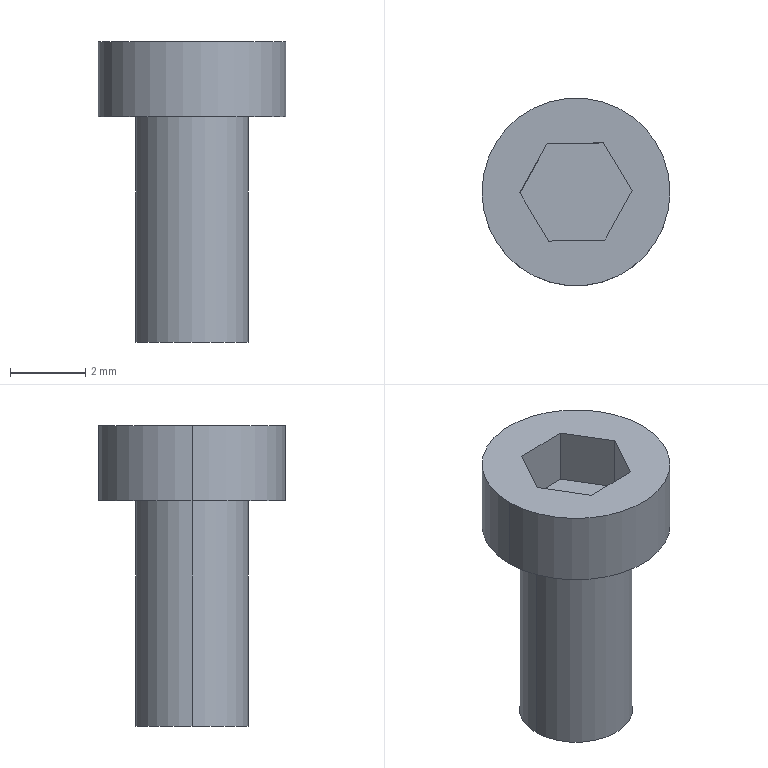Part | SolidWorks | features Cut 1, Extrusion 1, ICE 1 | 1 solid | 14 faces | box 5 x 5 x 8 mm | volume 72.989 mm3 | plane 10 | cylinder 4 | commonest cylinder face diameters 3 x2 5 x2
STEP:
#1=CARTESIAN_POINT('',(2.5,0.,2.));
#2=VERTEX_POINT('',#1);
#3=CARTESIAN_POINT('',(-2.5,0.,2.));
#4=VERTEX_POINT('',#3);
#5=CARTESIAN_POINT('',(0.,0.,2.));
#6=DIRECTION('',(0.,0.,1.));
#7=DIRECTION('',(1.,0.,0.));
#8=AXIS2_PLACEMENT_3D('',#5,#6,#7);
#9=CIRCLE('',#8,2.5);
#10=EDGE_CURVE('',#2,#4,#9,.T.);
#11=ORIENTED_EDGE('',*,*,#10,.F.);
#12=CARTESIAN_POINT('',(2.5,0.,0.));
#13=VERTEX_POINT('',#12);
#14=CARTESIAN_POINT('',(2.5,0.,2.));
#15=DIRECTION('',(0.,0.,-1.));
#16=VECTOR('',#15,1000.);
#17=LINE('',#14,#16);
#18=EDGE_CURVE('',#2,#13,#17,.T.);
#19=ORIENTED_EDGE('',*,*,#18,.T.);
#20=CARTESIAN_POINT('',(-2.5,0.,0.));
#21=VERTEX_POINT('',#20);
#22=CARTESIAN_POINT('',(0.,0.,0.));
#23=DIRECTION('',(0.,0.,1.));
#24=DIRECTION('',(1.,0.,0.));
#25=AXIS2_PLACEMENT_3D('',#22,#23,#24);
#26=CIRCLE('',#25,2.5);
#27=EDGE_CURVE('',#13,#21,#26,.T.);
#28=ORIENTED_EDGE('',*,*,#27,.T.);
#29=CARTESIAN_POINT('',(-2.5,0.,2.));
#30=DIRECTION('',(0.,0.,-1.));
#31=VECTOR('',#30,1000.);
#32=LINE('',#29,#31);
#33=EDGE_CURVE('',#4,#21,#32,.T.);
#34=ORIENTED_EDGE('',*,*,#33,.F.);
#35=EDGE_LOOP('',(#11,#19,#28,#34));
#36=FACE_OUTER_BOUND('',#35,.T.);
#37=CARTESIAN_POINT('',(0.,0.,2.));
#38=DIRECTION('',(0.,0.,-1.));
#39=DIRECTION('',(-1.,0.,0.));
#40=AXIS2_PLACEMENT_3D('',#37,#38,#39);
#41=CYLINDRICAL_SURFACE('',#40,2.5);
#42=ADVANCED_FACE('',(#36),#41,.T.);
#43=CARTESIAN_POINT('',(1.5,0.,-6.));
#44=VERTEX_POINT('',#43);
#45=CARTESIAN_POINT('',(-1.5,0.,-6.));
#46=VERTEX_POINT('',#45);
#47=CARTESIAN_POINT('',(0.,0.,-6.));
#48=DIRECTION('',(0.,0.,1.));
#49=DIRECTION('',(1.,0.,0.));
#50=AXIS2_PLACEMENT_3D('',#47,#48,#49);
#51=CIRCLE('',#50,1.5);
#52=EDGE_CURVE('',#44,#46,#51,.T.);
#53=ORIENTED_EDGE('',*,*,#52,.T.);
#54=CARTESIAN_POINT('',(-1.5,0.,0.));
#55=VERTEX_POINT('',#54);
#56=CARTESIAN_POINT('',(-1.5,0.,-6.));
#57=DIRECTION('',(0.,0.,1.));
#58=VECTOR('',#57,1000.);
#59=LINE('',#56,#58);
#60=EDGE_CURVE('',#46,#55,#59,.T.);
#61=ORIENTED_EDGE('',*,*,#60,.T.);
#62=CARTESIAN_POINT('',(1.5,0.,0.));
#63=VERTEX_POINT('',#62);
#64=CARTESIAN_POINT('',(0.,0.,0.));
#65=DIRECTION('',(0.,0.,1.));
#66=DIRECTION('',(1.,0.,0.));
#67=AXIS2_PLACEMENT_3D('',#64,#65,#66);
#68=CIRCLE('',#67,1.5);
#69=EDGE_CURVE('',#63,#55,#68,.T.);
#70=ORIENTED_EDGE('',*,*,#69,.F.);
#71=CARTESIAN_POINT('',(1.5,0.,-6.));
#72=DIRECTION('',(0.,0.,1.));
#73=VECTOR('',#72,1000.);
#74=LINE('',#71,#73);
#75=EDGE_CURVE('',#44,#63,#74,.T.);
#76=ORIENTED_EDGE('',*,*,#75,.F.);
#77=EDGE_LOOP('',(#53,#61,#70,#76));
#78=FACE_OUTER_BOUND('',#77,.T.);
#79=CARTESIAN_POINT('',(0.,0.,-6.));
#80=DIRECTION('',(0.,0.,1.));
#81=DIRECTION('',(1.,0.,0.));
#82=AXIS2_PLACEMENT_3D('',#79,#80,#81);
#83=CYLINDRICAL_SURFACE('',#82,1.5);
#84=ADVANCED_FACE('',(#78),#83,.T.);
#85=ORIENTED_EDGE('',*,*,#60,.F.);
#86=CARTESIAN_POINT('',(0.,0.,-6.));
#87=DIRECTION('',(0.,0.,1.));
#88=DIRECTION('',(1.,0.,0.));
#89=AXIS2_PLACEMENT_3D('',#86,#87,#88);
#90=CIRCLE('',#89,1.5);
#91=EDGE_CURVE('',#46,#44,#90,.T.);
#92=ORIENTED_EDGE('',*,*,#91,.T.);
#93=ORIENTED_EDGE('',*,*,#75,.T.);
#94=CARTESIAN_POINT('',(0.,0.,0.));
#95=DIRECTION('',(0.,0.,1.));
#96=DIRECTION('',(1.,0.,0.));
#97=AXIS2_PLACEMENT_3D('',#94,#95,#96);
#98=CIRCLE('',#97,1.5);
#99=EDGE_CURVE('',#55,#63,#98,.T.);
#100=ORIENTED_EDGE('',*,*,#99,.F.);
#101=EDGE_LOOP('',(#85,#92,#93,#100));
#102=FACE_OUTER_BOUND('',#101,.T.);
#103=CARTESIAN_POINT('',(0.,0.,-6.));
#104=DIRECTION('',(0.,0.,1.));
#105=DIRECTION('',(1.,0.,0.));
#106=AXIS2_PLACEMENT_3D('',#103,#104,#105);
#107=CYLINDRICAL_SURFACE('',#106,1.5);
#108=ADVANCED_FACE('',(#102),#107,.T.);
#109=ORIENTED_EDGE('',*,*,#52,.F.);
#110=ORIENTED_EDGE('',*,*,#91,.F.);
#111=EDGE_LOOP('',(#109,#110));
#112=FACE_OUTER_BOUND('',#111,.T.);
#113=CARTESIAN_POINT('',(0.,0.,-6.));
#114=DIRECTION('',(0.,0.,1.));
#115=DIRECTION('',(1.,0.,0.));
#116=AXIS2_PLACEMENT_3D('',#113,#114,#115);
#117=PLANE('',#116);
#118=ADVANCED_FACE('',(#112),#117,.F.);
#119=ORIENTED_EDGE('',*,*,#18,.F.);
#120=CARTESIAN_POINT('',(0.,0.,2.));
#121=DIRECTION('',(0.,0.,1.));
#122=DIRECTION('',(1.,0.,0.));
#123=AXIS2_PLACEMENT_3D('',#120,#121,#122);
#124=CIRCLE('',#123,2.5);
#125=EDGE_CURVE('',#4,#2,#124,.T.);
#126=ORIENTED_EDGE('',*,*,#125,.F.);
#127=ORIENTED_EDGE('',*,*,#33,.T.);
#128=CARTESIAN_POINT('',(0.,0.,0.));
#129=DIRECTION('',(0.,0.,1.));
#130=DIRECTION('',(1.,0.,0.));
#131=AXIS2_PLACEMENT_3D('',#128,#129,#130);
#132=CIRCLE('',#131,2.5);
#133=EDGE_CURVE('',#21,#13,#132,.T.);
#134=ORIENTED_EDGE('',*,*,#133,.T.);
#135=EDGE_LOOP('',(#119,#126,#127,#134));
#136=FACE_OUTER_BOUND('',#135,.T.);
#137=CARTESIAN_POINT('',(0.,0.,2.));
#138=DIRECTION('',(0.,0.,-1.));
#139=DIRECTION('',(-1.,0.,0.));
#140=AXIS2_PLACEMENT_3D('',#137,#138,#139);
#141=CYLINDRICAL_SURFACE('',#140,2.5);
#142=ADVANCED_FACE('',(#136),#141,.T.);
#143=CARTESIAN_POINT('',(1.493,0.02809,2.));
#144=VERTEX_POINT('',#143);
#145=CARTESIAN_POINT('',(0.7223,1.307,2.));
#146=VERTEX_POINT('',#145);
#147=CARTESIAN_POINT('',(1.493,0.02809,2.));
#148=DIRECTION('',(-0.5162,0.8565,0.));
#149=VECTOR('',#148,1000.);
#150=LINE('',#147,#149);
#151=EDGE_CURVE('',#144,#146,#150,.T.);
#152=ORIENTED_EDGE('',*,*,#151,.F.);
#153=CARTESIAN_POINT('',(0.7709,-1.279,2.));
#154=VERTEX_POINT('',#153);
#155=CARTESIAN_POINT('',(0.7709,-1.279,2.));
#156=DIRECTION('',(0.4836,0.8753,0.));
#157=VECTOR('',#156,1000.);
#158=LINE('',#155,#157);
#159=EDGE_CURVE('',#154,#144,#158,.T.);
#160=ORIENTED_EDGE('',*,*,#159,.F.);
#161=CARTESIAN_POINT('',(-0.7223,-1.307,2.));
#162=VERTEX_POINT('',#161);
#163=CARTESIAN_POINT('',(-0.7223,-1.307,2.));
#164=DIRECTION('',(0.9998,0.01881,0.));
#165=VECTOR('',#164,1000.);
#166=LINE('',#163,#165);
#167=EDGE_CURVE('',#162,#154,#166,.T.);
#168=ORIENTED_EDGE('',*,*,#167,.F.);
#169=CARTESIAN_POINT('',(-1.493,-0.02809,2.));
#170=VERTEX_POINT('',#169);
#171=CARTESIAN_POINT('',(-1.493,-0.02809,2.));
#172=DIRECTION('',(0.5162,-0.8565,0.));
#173=VECTOR('',#172,1000.);
#174=LINE('',#171,#173);
#175=EDGE_CURVE('',#170,#162,#174,.T.);
#176=ORIENTED_EDGE('',*,*,#175,.F.);
#177=CARTESIAN_POINT('',(-0.7709,1.279,2.));
#178=VERTEX_POINT('',#177);
#179=CARTESIAN_POINT('',(-0.7709,1.279,2.));
#180=DIRECTION('',(-0.4836,-0.8753,0.));
#181=VECTOR('',#180,1000.);
#182=LINE('',#179,#181);
#183=EDGE_CURVE('',#178,#170,#182,.T.);
#184=ORIENTED_EDGE('',*,*,#183,.F.);
#185=CARTESIAN_POINT('',(0.7223,1.307,2.));
#186=DIRECTION('',(-0.9998,-0.01881,0.));
#187=VECTOR('',#186,1000.);
#188=LINE('',#185,#187);
#189=EDGE_CURVE('',#146,#178,#188,.T.);
#190=ORIENTED_EDGE('',*,*,#189,.F.);
#191=EDGE_LOOP('',(#152,#160,#168,#176,#184,#190));
#192=FACE_BOUND('',#191,.T.);
#193=ORIENTED_EDGE('',*,*,#125,.T.);
#194=ORIENTED_EDGE('',*,*,#10,.T.);
#195=EDGE_LOOP('',(#193,#194));
#196=FACE_OUTER_BOUND('',#195,.T.);
#197=CARTESIAN_POINT('',(0.,0.,2.));
#198=DIRECTION('',(0.,0.,1.));
#199=DIRECTION('',(1.,0.,0.));
#200=AXIS2_PLACEMENT_3D('',#197,#198,#199);
#201=PLANE('',#200);
#202=ADVANCED_FACE('',(#192,#196),#201,.T.);
#203=ORIENTED_EDGE('',*,*,#69,.T.);
#204=ORIENTED_EDGE('',*,*,#99,.T.);
#205=EDGE_LOOP('',(#203,#204));
#206=FACE_BOUND('',#205,.T.);
#207=ORIENTED_EDGE('',*,*,#133,.F.);
#208=ORIENTED_EDGE('',*,*,#27,.F.);
#209=EDGE_LOOP('',(#207,#208));
#210=FACE_OUTER_BOUND('',#209,.T.);
#211=CARTESIAN_POINT('',(0.,0.,0.));
#212=DIRECTION('',(0.,0.,1.));
#213=DIRECTION('',(1.,0.,0.));
#214=AXIS2_PLACEMENT_3D('',#211,#212,#213);
#215=PLANE('',#214);
#216=ADVANCED_FACE('',(#206,#210),#215,.F.);
#217=ORIENTED_EDGE('',*,*,#151,.T.);
#218=CARTESIAN_POINT('',(0.7223,1.307,0.5));
#219=VERTEX_POINT('',#218);
#220=CARTESIAN_POINT('',(0.7223,1.307,0.5));
#221=DIRECTION('',(0.,0.,1.));
#222=VECTOR('',#221,1000.);
#223=LINE('',#220,#222);
#224=EDGE_CURVE('',#219,#146,#223,.T.);
#225=ORIENTED_EDGE('',*,*,#224,.F.);
#226=CARTESIAN_POINT('',(1.493,0.02809,0.5));
#227=VERTEX_POINT('',#226);
#228=CARTESIAN_POINT('',(1.493,0.02809,0.5));
#229=DIRECTION('',(-0.5162,0.8565,0.));
#230=VECTOR('',#229,1000.);
#231=LINE('',#228,#230);
#232=EDGE_CURVE('',#227,#219,#231,.T.);
#233=ORIENTED_EDGE('',*,*,#232,.F.);
#234=CARTESIAN_POINT('',(1.493,0.02809,0.5));
#235=DIRECTION('',(0.,0.,1.));
#236=VECTOR('',#235,1000.);
#237=LINE('',#234,#236);
#238=EDGE_CURVE('',#227,#144,#237,.T.);
#239=ORIENTED_EDGE('',*,*,#238,.T.);
#240=EDGE_LOOP('',(#217,#225,#233,#239));
#241=FACE_OUTER_BOUND('',#240,.T.);
#242=CARTESIAN_POINT('',(1.493,0.02809,0.5));
#243=DIRECTION('',(0.8565,0.5162,0.));
#244=DIRECTION('',(-0.5162,0.8565,0.));
#245=AXIS2_PLACEMENT_3D('',#242,#243,#244);
#246=PLANE('',#245);
#247=ADVANCED_FACE('',(#241),#246,.F.);
#248=ORIENTED_EDGE('',*,*,#159,.T.);
#249=ORIENTED_EDGE('',*,*,#238,.F.);
#250=CARTESIAN_POINT('',(0.7709,-1.279,0.5));
#251=VERTEX_POINT('',#250);
#252=CARTESIAN_POINT('',(0.7709,-1.279,0.5));
#253=DIRECTION('',(0.4836,0.8753,0.));
#254=VECTOR('',#253,1000.);
#255=LINE('',#252,#254);
#256=EDGE_CURVE('',#251,#227,#255,.T.);
#257=ORIENTED_EDGE('',*,*,#256,.F.);
#258=CARTESIAN_POINT('',(0.7709,-1.279,0.5));
#259=DIRECTION('',(0.,0.,1.));
#260=VECTOR('',#259,1000.);
#261=LINE('',#258,#260);
#262=EDGE_CURVE('',#251,#154,#261,.T.);
#263=ORIENTED_EDGE('',*,*,#262,.T.);
#264=EDGE_LOOP('',(#248,#249,#257,#263));
#265=FACE_OUTER_BOUND('',#264,.T.);
#266=CARTESIAN_POINT('',(0.7709,-1.279,0.5));
#267=DIRECTION('',(0.8753,-0.4836,0.));
#268=DIRECTION('',(0.4836,0.8753,0.));
#269=AXIS2_PLACEMENT_3D('',#266,#267,#268);
#270=PLANE('',#269);
#271=ADVANCED_FACE('',(#265),#270,.F.);
#272=ORIENTED_EDGE('',*,*,#167,.T.);
#273=ORIENTED_EDGE('',*,*,#262,.F.);
#274=CARTESIAN_POINT('',(-0.7223,-1.307,0.5));
#275=VERTEX_POINT('',#274);
#276=CARTESIAN_POINT('',(-0.7223,-1.307,0.5));
#277=DIRECTION('',(0.9998,0.01881,0.));
#278=VECTOR('',#277,1000.);
#279=LINE('',#276,#278);
#280=EDGE_CURVE('',#275,#251,#279,.T.);
#281=ORIENTED_EDGE('',*,*,#280,.F.);
#282=CARTESIAN_POINT('',(-0.7223,-1.307,0.5));
#283=DIRECTION('',(0.,0.,1.));
#284=VECTOR('',#283,1000.);
#285=LINE('',#282,#284);
#286=EDGE_CURVE('',#275,#162,#285,.T.);
#287=ORIENTED_EDGE('',*,*,#286,.T.);
#288=EDGE_LOOP('',(#272,#273,#281,#287));
#289=FACE_OUTER_BOUND('',#288,.T.);
#290=CARTESIAN_POINT('',(-0.7223,-1.307,0.5));
#291=DIRECTION('',(0.01881,-0.9998,0.));
#292=DIRECTION('',(0.9998,0.01881,0.));
#293=AXIS2_PLACEMENT_3D('',#290,#291,#292);
#294=PLANE('',#293);
#295=ADVANCED_FACE('',(#289),#294,.F.);
#296=ORIENTED_EDGE('',*,*,#175,.T.);
#297=ORIENTED_EDGE('',*,*,#286,.F.);
#298=CARTESIAN_POINT('',(-1.493,-0.02809,0.5));
#299=VERTEX_POINT('',#298);
#300=CARTESIAN_POINT('',(-1.493,-0.02809,0.5));
#301=DIRECTION('',(0.5162,-0.8565,0.));
#302=VECTOR('',#301,1000.);
#303=LINE('',#300,#302);
#304=EDGE_CURVE('',#299,#275,#303,.T.);
#305=ORIENTED_EDGE('',*,*,#304,.F.);
#306=CARTESIAN_POINT('',(-1.493,-0.02809,0.5));
#307=DIRECTION('',(0.,0.,1.));
#308=VECTOR('',#307,1000.);
#309=LINE('',#306,#308);
#310=EDGE_CURVE('',#299,#170,#309,.T.);
#311=ORIENTED_EDGE('',*,*,#310,.T.);
#312=EDGE_LOOP('',(#296,#297,#305,#311));
#313=FACE_OUTER_BOUND('',#312,.T.);
#314=CARTESIAN_POINT('',(-1.493,-0.02809,0.5));
#315=DIRECTION('',(-0.8565,-0.5162,0.));
#316=DIRECTION('',(0.5162,-0.8565,0.));
#317=AXIS2_PLACEMENT_3D('',#314,#315,#316);
#318=PLANE('',#317);
#319=ADVANCED_FACE('',(#313),#318,.F.);
#320=ORIENTED_EDGE('',*,*,#183,.T.);
#321=ORIENTED_EDGE('',*,*,#310,.F.);
#322=CARTESIAN_POINT('',(-0.7709,1.279,0.5));
#323=VERTEX_POINT('',#322);
#324=CARTESIAN_POINT('',(-0.7709,1.279,0.5));
#325=DIRECTION('',(-0.4836,-0.8753,0.));
#326=VECTOR('',#325,1000.);
#327=LINE('',#324,#326);
#328=EDGE_CURVE('',#323,#299,#327,.T.);
#329=ORIENTED_EDGE('',*,*,#328,.F.);
#330=CARTESIAN_POINT('',(-0.7709,1.279,0.5));
#331=DIRECTION('',(0.,0.,1.));
#332=VECTOR('',#331,1000.);
#333=LINE('',#330,#332);
#334=EDGE_CURVE('',#323,#178,#333,.T.);
#335=ORIENTED_EDGE('',*,*,#334,.T.);
#336=EDGE_LOOP('',(#320,#321,#329,#335));
#337=FACE_OUTER_BOUND('',#336,.T.);
#338=CARTESIAN_POINT('',(-0.7709,1.279,0.5));
#339=DIRECTION('',(-0.8753,0.4836,0.));
#340=DIRECTION('',(-0.4836,-0.8753,0.));
#341=AXIS2_PLACEMENT_3D('',#338,#339,#340);
#342=PLANE('',#341);
#343=ADVANCED_FACE('',(#337),#342,.F.);
#344=ORIENTED_EDGE('',*,*,#189,.T.);
#345=ORIENTED_EDGE('',*,*,#334,.F.);
#346=CARTESIAN_POINT('',(0.7223,1.307,0.5));
#347=DIRECTION('',(-0.9998,-0.01881,0.));
#348=VECTOR('',#347,1000.);
#349=LINE('',#346,#348);
#350=EDGE_CURVE('',#219,#323,#349,.T.);
#351=ORIENTED_EDGE('',*,*,#350,.F.);
#352=ORIENTED_EDGE('',*,*,#224,.T.);
#353=EDGE_LOOP('',(#344,#345,#351,#352));
#354=FACE_OUTER_BOUND('',#353,.T.);
#355=CARTESIAN_POINT('',(0.7223,1.307,0.5));
#356=DIRECTION('',(-0.01881,0.9998,0.));
#357=DIRECTION('',(-0.9998,-0.01881,0.));
#358=AXIS2_PLACEMENT_3D('',#355,#356,#357);
#359=PLANE('',#358);
#360=ADVANCED_FACE('',(#354),#359,.F.);
#361=ORIENTED_EDGE('',*,*,#232,.T.);
#362=ORIENTED_EDGE('',*,*,#350,.T.);
#363=ORIENTED_EDGE('',*,*,#328,.T.);
#364=ORIENTED_EDGE('',*,*,#304,.T.);
#365=ORIENTED_EDGE('',*,*,#280,.T.);
#366=ORIENTED_EDGE('',*,*,#256,.T.);
#367=EDGE_LOOP('',(#361,#362,#363,#364,#365,#366));
#368=FACE_OUTER_BOUND('',#367,.T.);
#369=CARTESIAN_POINT('',(0.,0.,0.5));
#370=DIRECTION('',(0.,0.,1.));
#371=DIRECTION('',(1.,0.,0.));
#372=AXIS2_PLACEMENT_3D('',#369,#370,#371);
#373=PLANE('',#372);
#374=ADVANCED_FACE('',(#368),#373,.T.);
#375=CLOSED_SHELL('',(#42,#84,#108,#118,#142,#202,#216,#247,#271,#295,#319,#343,#360,#374));
#376=MANIFOLD_SOLID_BREP('',#375);
#377=CARTESIAN_POINT('',(0.,0.,0.));
#378=DIRECTION('',(0.,0.,1.));
#379=DIRECTION('',(1.,0.,0.));
#380=AXIS2_PLACEMENT_3D('',#377,#378,#379);
#381=(LENGTH_UNIT()NAMED_UNIT(*)SI_UNIT(.MILLI.,.METRE.));
#382=UNCERTAINTY_MEASURE_WITH_UNIT(LENGTH_MEASURE(0.00001),#381,'','');
#383=(NAMED_UNIT(*)PLANE_ANGLE_UNIT()SI_UNIT($,.RADIAN.));
#384=(NAMED_UNIT(*)SI_UNIT($,.STERADIAN.)SOLID_ANGLE_UNIT());
#385=(GEOMETRIC_REPRESENTATION_CONTEXT(3)GLOBAL_UNCERTAINTY_ASSIGNED_CONTEXT((#382))GLOBAL_UNIT_ASSIGNED_CONTEXT((#381,#383,#384))REPRESENTATION_CONTEXT('',''));
#386=ADVANCED_BREP_SHAPE_REPRESENTATION('',(#376,#380),#385);